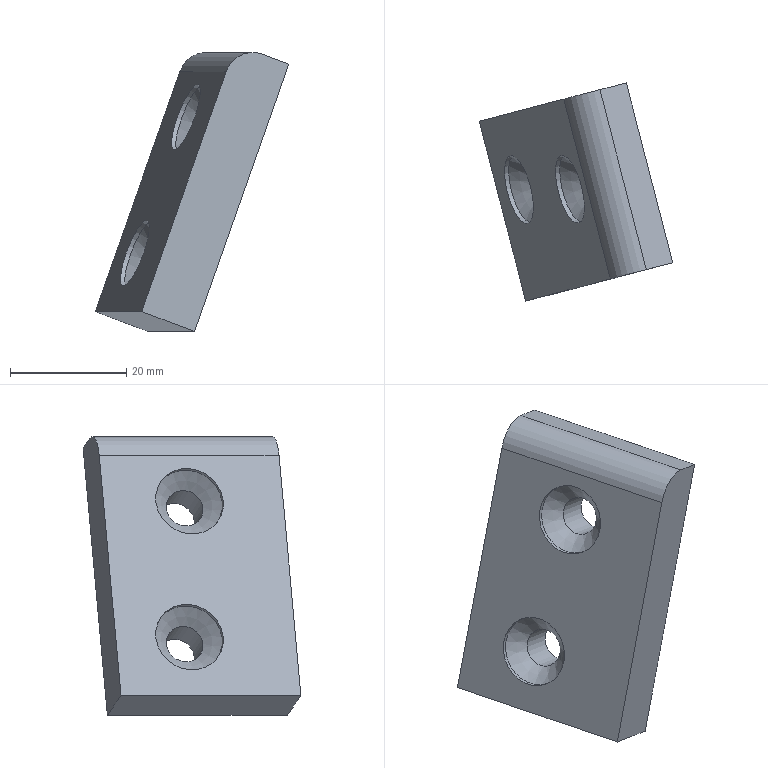Part | STEP file | 车灯-后视镜_id274_x_t | 1 solid | 13 faces | box 33.319 x 37.519 x 48.057 mm | volume 14519 mm3 | plane 6 | cylinder 5 | cone 2 | commonest cylinder face diameters 6.5 x2 12 x2 10 x1
STEP:
#1=CARTESIAN_POINT('',(-151.622,-120.288,-3.567));
#2=VERTEX_POINT('',#1);
#3=CARTESIAN_POINT('',(-143.629,-151.273,-3.567));
#4=VERTEX_POINT('',#3);
#5=CARTESIAN_POINT('',(-142.63,-155.147,-3.567));
#6=DIRECTION('',(0.2498,-0.9683,0.));
#7=VECTOR('',#6,1.);
#8=LINE('',#5,#7);
#9=EDGE_CURVE('',#2,#4,#8,.T.);
#10=ORIENTED_EDGE('',*,*,#9,.T.);
#11=CARTESIAN_POINT('',(-152.729,-153.62,-0.1472));
#12=VERTEX_POINT('',#11);
#13=CARTESIAN_POINT('',(-143.629,-151.273,-3.567));
#14=DIRECTION('',(-0.9099,-0.2347,0.342));
#15=VECTOR('',#14,1.);
#16=LINE('',#13,#15);
#17=EDGE_CURVE('',#4,#12,#16,.T.);
#18=ORIENTED_EDGE('',*,*,#17,.T.);
#19=CARTESIAN_POINT('',(-160.721,-122.635,-0.1472));
#20=VERTEX_POINT('',#19);
#21=CARTESIAN_POINT('',(-151.73,-157.494,-0.1472));
#22=DIRECTION('',(0.2498,-0.9683,0.));
#23=VECTOR('',#22,1.);
#24=LINE('',#21,#23);
#25=EDGE_CURVE('',#20,#12,#24,.T.);
#26=ORIENTED_EDGE('',*,*,#25,.F.);
#27=CARTESIAN_POINT('',(-151.622,-120.288,-3.567));
#28=DIRECTION('',(-0.9099,-0.2347,0.342));
#29=VECTOR('',#28,1.);
#30=LINE('',#27,#29);
#31=EDGE_CURVE('',#2,#20,#30,.T.);
#32=ORIENTED_EDGE('',*,*,#31,.F.);
#33=EDGE_LOOP('',(#10,#18,#26,#32));
#34=FACE_OUTER_BOUND('',#33,.T.);
#35=CARTESIAN_POINT('',(-142.63,-155.147,-3.567));
#36=DIRECTION('',(-0.3312,-0.08542,-0.9397));
#37=DIRECTION('',(-0.9431,0.,0.3324));
#38=AXIS2_PLACEMENT_3D('',#35,#36,#37);
#39=PLANE('',#38);
#40=ADVANCED_FACE('',(#34),#39,.T.);
#41=CARTESIAN_POINT('',(-143.651,-132.082,9.546));
#42=VERTEX_POINT('',#41);
#43=CARTESIAN_POINT('',(-144.794,-132.082,6.504));
#44=DIRECTION('',(0.9099,0.2347,-0.342));
#45=DIRECTION('',(0.3518,0.,0.9361));
#46=AXIS2_PLACEMENT_3D('',#43,#44,#45);
#47=CIRCLE('',#46,3.25);
#48=EDGE_CURVE('',#42,#42,#47,.T.);
#49=ORIENTED_EDGE('',*,*,#48,.F.);
#50=EDGE_LOOP('',(#49));
#51=FACE_BOUND('',#50,.T.);
#52=CARTESIAN_POINT('',(-134.854,-132.082,32.948));
#53=VERTEX_POINT('',#52);
#54=CARTESIAN_POINT('',(-135.998,-132.082,29.905));
#55=DIRECTION('',(0.9099,0.2347,-0.342));
#56=DIRECTION('',(0.3518,0.,0.9361));
#57=AXIS2_PLACEMENT_3D('',#54,#55,#56);
#58=CIRCLE('',#57,3.25);
#59=EDGE_CURVE('',#53,#53,#58,.T.);
#60=ORIENTED_EDGE('',*,*,#59,.F.);
#61=EDGE_LOOP('',(#60));
#62=FACE_BOUND('',#61,.T.);
#63=CARTESIAN_POINT('',(-127.402,-147.088,42.478));
#64=VERTEX_POINT('',#63);
#65=CARTESIAN_POINT('',(-143.629,-151.273,-3.567));
#66=DIRECTION('',(0.3312,0.08542,0.9397));
#67=VECTOR('',#66,1.);
#68=LINE('',#65,#67);
#69=EDGE_CURVE('',#4,#64,#68,.T.);
#70=ORIENTED_EDGE('',*,*,#69,.F.);
#71=ORIENTED_EDGE('',*,*,#9,.F.);
#72=CARTESIAN_POINT('',(-135.394,-116.102,42.478));
#73=VERTEX_POINT('',#72);
#74=CARTESIAN_POINT('',(-151.622,-120.288,-3.567));
#75=DIRECTION('',(0.3312,0.08542,0.9397));
#76=VECTOR('',#75,1.);
#77=LINE('',#74,#76);
#78=EDGE_CURVE('',#2,#73,#77,.T.);
#79=ORIENTED_EDGE('',*,*,#78,.T.);
#80=CARTESIAN_POINT('',(-126.403,-150.961,42.478));
#81=DIRECTION('',(-0.2498,0.9683,0.));
#82=VECTOR('',#81,1.);
#83=LINE('',#80,#82);
#84=EDGE_CURVE('',#64,#73,#83,.T.);
#85=ORIENTED_EDGE('',*,*,#84,.F.);
#86=EDGE_LOOP('',(#70,#71,#79,#85));
#87=FACE_BOUND('',#86,.T.);
#88=CARTESIAN_POINT('',(-142.63,-155.147,-3.567));
#89=DIRECTION('',(-0.9099,-0.2347,0.342));
#90=DIRECTION('',(0.3518,0.,0.9361));
#91=AXIS2_PLACEMENT_3D('',#88,#89,#90);
#92=PLANE('',#91);
#93=ADVANCED_FACE('',(#51,#62,#87),#92,.F.);
#94=CARTESIAN_POINT('',(-151.782,-134.429,15.541));
#95=VERTEX_POINT('',#94);
#96=CARTESIAN_POINT('',(-153.893,-134.429,9.924));
#97=DIRECTION('',(0.9099,0.2347,-0.342));
#98=DIRECTION('',(0.3518,0.,0.9361));
#99=AXIS2_PLACEMENT_3D('',#96,#97,#98);
#100=CIRCLE('',#99,6.);
#101=EDGE_CURVE('',#95,#95,#100,.T.);
#102=ORIENTED_EDGE('',*,*,#101,.T.);
#103=EDGE_LOOP('',(#102));
#104=FACE_BOUND('',#103,.T.);
#105=CARTESIAN_POINT('',(-142.986,-134.429,38.942));
#106=VERTEX_POINT('',#105);
#107=CARTESIAN_POINT('',(-145.097,-134.429,33.326));
#108=DIRECTION('',(0.9099,0.2347,-0.342));
#109=DIRECTION('',(0.3518,0.,0.9361));
#110=AXIS2_PLACEMENT_3D('',#107,#108,#109);
#111=CIRCLE('',#110,6.);
#112=EDGE_CURVE('',#106,#106,#111,.T.);
#113=ORIENTED_EDGE('',*,*,#112,.T.);
#114=EDGE_LOOP('',(#113));
#115=FACE_BOUND('',#114,.T.);
#116=CARTESIAN_POINT('',(-138.157,-149.862,41.199));
#117=VERTEX_POINT('',#116);
#118=CARTESIAN_POINT('',(-152.729,-153.62,-0.1472));
#119=DIRECTION('',(0.3312,0.08542,0.9397));
#120=VECTOR('',#119,1.);
#121=LINE('',#118,#120);
#122=EDGE_CURVE('',#12,#117,#121,.T.);
#123=ORIENTED_EDGE('',*,*,#122,.T.);
#124=CARTESIAN_POINT('',(-146.149,-118.876,41.199));
#125=VERTEX_POINT('',#124);
#126=CARTESIAN_POINT('',(-137.158,-153.735,41.199));
#127=DIRECTION('',(-0.2498,0.9683,0.));
#128=VECTOR('',#127,1.);
#129=LINE('',#126,#128);
#130=EDGE_CURVE('',#117,#125,#129,.T.);
#131=ORIENTED_EDGE('',*,*,#130,.T.);
#132=CARTESIAN_POINT('',(-160.721,-122.635,-0.1472));
#133=DIRECTION('',(0.3312,0.08542,0.9397));
#134=VECTOR('',#133,1.);
#135=LINE('',#132,#134);
#136=EDGE_CURVE('',#20,#125,#135,.T.);
#137=ORIENTED_EDGE('',*,*,#136,.F.);
#138=ORIENTED_EDGE('',*,*,#25,.T.);
#139=EDGE_LOOP('',(#123,#131,#137,#138));
#140=FACE_BOUND('',#139,.T.);
#141=CARTESIAN_POINT('',(-151.73,-157.494,-0.1472));
#142=DIRECTION('',(-0.9099,-0.2347,0.342));
#143=DIRECTION('',(0.3518,0.,0.9361));
#144=AXIS2_PLACEMENT_3D('',#141,#142,#143);
#145=PLANE('',#144);
#146=ADVANCED_FACE('',(#104,#115,#140),#145,.T.);
#147=CARTESIAN_POINT('',(-139.944,-117.275,44.188));
#148=VERTEX_POINT('',#147);
#149=CARTESIAN_POINT('',(-139.944,-117.275,44.188));
#150=DIRECTION('',(-0.9099,-0.2347,0.342));
#151=VECTOR('',#150,1.);
#152=LINE('',#149,#151);
#153=EDGE_CURVE('',#73,#148,#152,.T.);
#154=ORIENTED_EDGE('',*,*,#153,.T.);
#155=CARTESIAN_POINT('',(-131.951,-148.261,44.188));
#156=VERTEX_POINT('',#155);
#157=CARTESIAN_POINT('',(-130.952,-152.134,44.188));
#158=DIRECTION('',(0.2498,-0.9683,0.));
#159=VECTOR('',#158,1.);
#160=LINE('',#157,#159);
#161=EDGE_CURVE('',#148,#156,#160,.T.);
#162=ORIENTED_EDGE('',*,*,#161,.T.);
#163=CARTESIAN_POINT('',(-127.402,-147.088,42.478));
#164=DIRECTION('',(0.9099,0.2347,-0.342));
#165=VECTOR('',#164,1.);
#166=LINE('',#163,#165);
#167=EDGE_CURVE('',#156,#64,#166,.T.);
#168=ORIENTED_EDGE('',*,*,#167,.T.);
#169=ORIENTED_EDGE('',*,*,#84,.T.);
#170=EDGE_LOOP('',(#154,#162,#168,#169));
#171=FACE_OUTER_BOUND('',#170,.T.);
#172=CARTESIAN_POINT('',(-126.403,-150.961,42.478));
#173=DIRECTION('',(0.3312,0.08542,0.9397));
#174=DIRECTION('',(0.9431,0.,-0.3324));
#175=AXIS2_PLACEMENT_3D('',#172,#173,#174);
#176=PLANE('',#175);
#177=ADVANCED_FACE('',(#171),#176,.T.);
#178=ORIENTED_EDGE('',*,*,#136,.T.);
#179=CARTESIAN_POINT('',(-141.6,-117.702,39.489));
#180=DIRECTION('',(-0.2498,0.9683,0.));
#181=DIRECTION('',(0.9683,0.2498,0.));
#182=AXIS2_PLACEMENT_3D('',#179,#180,#181);
#183=CIRCLE('',#182,5.);
#184=EDGE_CURVE('',#125,#148,#183,.T.);
#185=ORIENTED_EDGE('',*,*,#184,.T.);
#186=ORIENTED_EDGE('',*,*,#153,.F.);
#187=ORIENTED_EDGE('',*,*,#78,.F.);
#188=ORIENTED_EDGE('',*,*,#31,.T.);
#189=EDGE_LOOP('',(#178,#185,#186,#187,#188));
#190=FACE_OUTER_BOUND('',#189,.T.);
#191=CARTESIAN_POINT('',(-140.312,-117.37,43.143));
#192=DIRECTION('',(0.2498,-0.9683,0.));
#193=DIRECTION('',(0.9683,0.2498,0.));
#194=AXIS2_PLACEMENT_3D('',#191,#192,#193);
#195=PLANE('',#194);
#196=ADVANCED_FACE('',(#190),#195,.F.);
#197=ORIENTED_EDGE('',*,*,#167,.F.);
#198=CARTESIAN_POINT('',(-133.607,-148.688,39.489));
#199=DIRECTION('',(0.2498,-0.9683,0.));
#200=DIRECTION('',(0.9683,0.2498,0.));
#201=AXIS2_PLACEMENT_3D('',#198,#199,#200);
#202=CIRCLE('',#201,5.);
#203=EDGE_CURVE('',#156,#117,#202,.T.);
#204=ORIENTED_EDGE('',*,*,#203,.T.);
#205=ORIENTED_EDGE('',*,*,#122,.F.);
#206=ORIENTED_EDGE('',*,*,#17,.F.);
#207=ORIENTED_EDGE('',*,*,#69,.T.);
#208=EDGE_LOOP('',(#197,#204,#205,#206,#207));
#209=FACE_OUTER_BOUND('',#208,.T.);
#210=CARTESIAN_POINT('',(-136.869,-149.53,44.853));
#211=DIRECTION('',(0.2498,-0.9683,0.));
#212=DIRECTION('',(0.9683,0.2498,0.));
#213=AXIS2_PLACEMENT_3D('',#210,#211,#212);
#214=PLANE('',#213);
#215=ADVANCED_FACE('',(#209),#214,.T.);
#216=ORIENTED_EDGE('',*,*,#203,.F.);
#217=ORIENTED_EDGE('',*,*,#161,.F.);
#218=ORIENTED_EDGE('',*,*,#184,.F.);
#219=ORIENTED_EDGE('',*,*,#130,.F.);
#220=EDGE_LOOP('',(#216,#217,#218,#219));
#221=FACE_OUTER_BOUND('',#220,.T.);
#222=CARTESIAN_POINT('',(-132.608,-152.562,39.489));
#223=DIRECTION('',(-0.2498,0.9683,0.));
#224=DIRECTION('',(-0.9683,-0.2498,0.));
#225=AXIS2_PLACEMENT_3D('',#222,#223,#224);
#226=CYLINDRICAL_SURFACE('',#225,5.);
#227=ADVANCED_FACE('',(#221),#226,.T.);
#228=CARTESIAN_POINT('',(-142.258,-134.241,38.668));
#229=VERTEX_POINT('',#228);
#230=CARTESIAN_POINT('',(-144.369,-134.241,33.052));
#231=DIRECTION('',(0.9099,0.2347,-0.342));
#232=DIRECTION('',(0.3518,0.,0.9361));
#233=AXIS2_PLACEMENT_3D('',#230,#231,#232);
#234=CIRCLE('',#233,6.);
#235=EDGE_CURVE('',#229,#229,#234,.T.);
#236=ORIENTED_EDGE('',*,*,#235,.T.);
#237=EDGE_LOOP('',(#236));
#238=FACE_BOUND('',#237,.T.);
#239=ORIENTED_EDGE('',*,*,#112,.F.);
#240=EDGE_LOOP('',(#239));
#241=FACE_BOUND('',#240,.T.);
#242=CARTESIAN_POINT('',(-144.642,-134.312,33.155));
#243=DIRECTION('',(0.9099,0.2347,-0.342));
#244=DIRECTION('',(-0.3518,0.,-0.9361));
#245=AXIS2_PLACEMENT_3D('',#242,#243,#244);
#246=CYLINDRICAL_SURFACE('',#245,6.);
#247=ADVANCED_FACE('',(#238,#241),#246,.F.);
#248=CARTESIAN_POINT('',(-140.723,-133.596,35.154));
#249=VERTEX_POINT('',#248);
#250=CARTESIAN_POINT('',(-141.867,-133.596,32.111));
#251=DIRECTION('',(0.9099,0.2347,-0.342));
#252=DIRECTION('',(0.3518,0.,0.9361));
#253=AXIS2_PLACEMENT_3D('',#250,#251,#252);
#254=CIRCLE('',#253,3.25);
#255=EDGE_CURVE('',#249,#249,#254,.T.);
#256=ORIENTED_EDGE('',*,*,#255,.T.);
#257=EDGE_LOOP('',(#256));
#258=FACE_BOUND('',#257,.T.);
#259=ORIENTED_EDGE('',*,*,#235,.F.);
#260=EDGE_LOOP('',(#259));
#261=FACE_BOUND('',#260,.T.);
#262=CARTESIAN_POINT('',(-144.369,-134.241,33.052));
#263=DIRECTION('',(-0.9099,-0.2347,0.342));
#264=DIRECTION('',(-0.3518,0.,-0.9361));
#265=AXIS2_PLACEMENT_3D('',#262,#263,#264);
#266=CONICAL_SURFACE('',#265,6.,45.);
#267=ADVANCED_FACE('',(#258,#261),#266,.F.);
#268=ORIENTED_EDGE('',*,*,#59,.T.);
#269=EDGE_LOOP('',(#268));
#270=FACE_BOUND('',#269,.T.);
#271=ORIENTED_EDGE('',*,*,#255,.F.);
#272=EDGE_LOOP('',(#271));
#273=FACE_BOUND('',#272,.T.);
#274=CARTESIAN_POINT('',(-141.639,-133.537,32.026));
#275=DIRECTION('',(0.9099,0.2347,-0.342));
#276=DIRECTION('',(-0.3518,0.,-0.9361));
#277=AXIS2_PLACEMENT_3D('',#274,#275,#276);
#278=CYLINDRICAL_SURFACE('',#277,3.25);
#279=ADVANCED_FACE('',(#270,#273),#278,.F.);
#280=CARTESIAN_POINT('',(-151.054,-134.241,15.267));
#281=VERTEX_POINT('',#280);
#282=CARTESIAN_POINT('',(-153.165,-134.241,9.651));
#283=DIRECTION('',(0.9099,0.2347,-0.342));
#284=DIRECTION('',(0.3518,0.,0.9361));
#285=AXIS2_PLACEMENT_3D('',#282,#283,#284);
#286=CIRCLE('',#285,6.);
#287=EDGE_CURVE('',#281,#281,#286,.T.);
#288=ORIENTED_EDGE('',*,*,#287,.T.);
#289=EDGE_LOOP('',(#288));
#290=FACE_BOUND('',#289,.T.);
#291=ORIENTED_EDGE('',*,*,#101,.F.);
#292=EDGE_LOOP('',(#291));
#293=FACE_BOUND('',#292,.T.);
#294=CARTESIAN_POINT('',(-153.438,-134.312,9.753));
#295=DIRECTION('',(0.9099,0.2347,-0.342));
#296=DIRECTION('',(-0.3518,0.,-0.9361));
#297=AXIS2_PLACEMENT_3D('',#294,#295,#296);
#298=CYLINDRICAL_SURFACE('',#297,6.);
#299=ADVANCED_FACE('',(#290,#293),#298,.F.);
#300=CARTESIAN_POINT('',(-149.519,-133.596,11.752));
#301=VERTEX_POINT('',#300);
#302=CARTESIAN_POINT('',(-150.663,-133.596,8.71));
#303=DIRECTION('',(0.9099,0.2347,-0.342));
#304=DIRECTION('',(0.3518,0.,0.9361));
#305=AXIS2_PLACEMENT_3D('',#302,#303,#304);
#306=CIRCLE('',#305,3.25);
#307=EDGE_CURVE('',#301,#301,#306,.T.);
#308=ORIENTED_EDGE('',*,*,#307,.T.);
#309=EDGE_LOOP('',(#308));
#310=FACE_BOUND('',#309,.T.);
#311=ORIENTED_EDGE('',*,*,#287,.F.);
#312=EDGE_LOOP('',(#311));
#313=FACE_BOUND('',#312,.T.);
#314=CARTESIAN_POINT('',(-153.165,-134.241,9.651));
#315=DIRECTION('',(-0.9099,-0.2347,0.342));
#316=DIRECTION('',(-0.3518,0.,-0.9361));
#317=AXIS2_PLACEMENT_3D('',#314,#315,#316);
#318=CONICAL_SURFACE('',#317,6.,45.);
#319=ADVANCED_FACE('',(#310,#313),#318,.F.);
#320=ORIENTED_EDGE('',*,*,#48,.T.);
#321=EDGE_LOOP('',(#320));
#322=FACE_BOUND('',#321,.T.);
#323=ORIENTED_EDGE('',*,*,#307,.F.);
#324=EDGE_LOOP('',(#323));
#325=FACE_BOUND('',#324,.T.);
#326=CARTESIAN_POINT('',(-150.435,-133.537,8.625));
#327=DIRECTION('',(0.9099,0.2347,-0.342));
#328=DIRECTION('',(-0.3518,0.,-0.9361));
#329=AXIS2_PLACEMENT_3D('',#326,#327,#328);
#330=CYLINDRICAL_SURFACE('',#329,3.25);
#331=ADVANCED_FACE('',(#322,#325),#330,.F.);
#332=CLOSED_SHELL('',(#40,#93,#146,#177,#196,#215,#227,#247,#267,#279,#299,#319,#331));
#333=MANIFOLD_SOLID_BREP('',#332);
#334=(LENGTH_UNIT()NAMED_UNIT(*)SI_UNIT(.MILLI.,.METRE.));
#335=UNCERTAINTY_MEASURE_WITH_UNIT(LENGTH_MEASURE(0.00002),#334,'','');
#336=(NAMED_UNIT(*)PLANE_ANGLE_UNIT()SI_UNIT($,.RADIAN.));
#337=PLANE_ANGLE_MEASURE_WITH_UNIT(PLANE_ANGLE_MEASURE(0.01745),#336);
#338=DIMENSIONAL_EXPONENTS(0.,0.,0.,0.,0.,0.,0.);
#339=(CONVERSION_BASED_UNIT('DEGREE',#337)NAMED_UNIT(#338)PLANE_ANGLE_UNIT());
#340=(NAMED_UNIT(*)SI_UNIT($,.STERADIAN.)SOLID_ANGLE_UNIT());
#341=(GEOMETRIC_REPRESENTATION_CONTEXT(3)GLOBAL_UNCERTAINTY_ASSIGNED_CONTEXT((#335))GLOBAL_UNIT_ASSIGNED_CONTEXT((#334,#339,#340))REPRESENTATION_CONTEXT('',''));
#342=ADVANCED_BREP_SHAPE_REPRESENTATION('',(#333),#341);